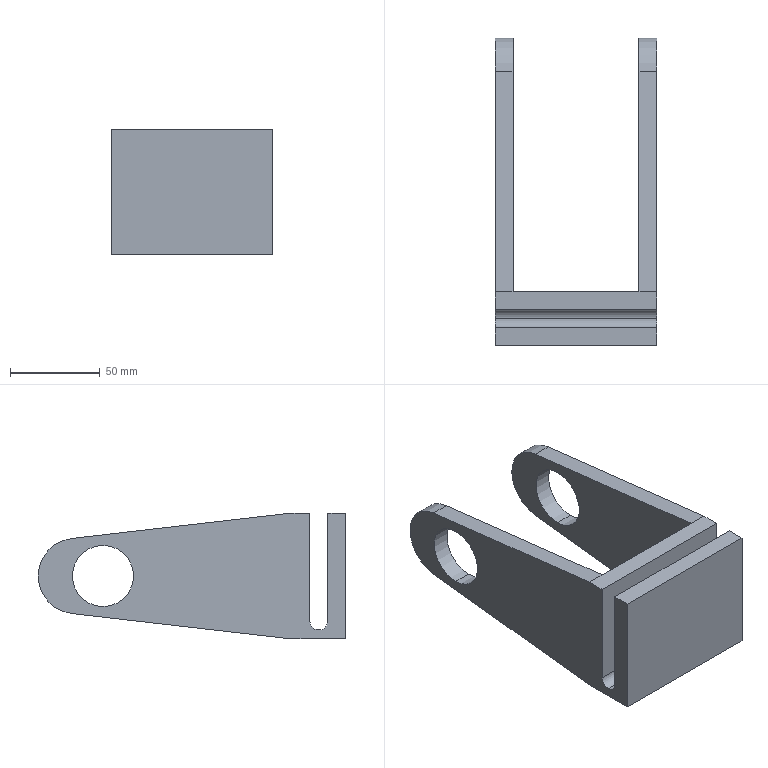Part | SolidWorks | features ICE 2, Extrusion 1, MirrorPattern 1 | 1 solid | 23 faces | box 90 x 171 x 70 mm | volume 261901 mm3 | plane 15 | cylinder 8 | commonest cylinder face diameters 34 x4 10 x2 42 x2
STEP:
#1=CARTESIAN_POINT('',(-45.,15.,-30.));
#2=VERTEX_POINT('',#1);
#3=CARTESIAN_POINT('',(-45.,20.,-25.));
#4=VERTEX_POINT('',#3);
#5=CARTESIAN_POINT('',(-45.,15.,-25.));
#6=DIRECTION('',(1.,0.,0.));
#7=DIRECTION('',(0.,0.,-1.));
#8=AXIS2_PLACEMENT_3D('',#5,#6,#7);
#9=CIRCLE('',#8,5.);
#10=EDGE_CURVE('',#2,#4,#9,.T.);
#11=ORIENTED_EDGE('',*,*,#10,.F.);
#12=CARTESIAN_POINT('',(45.,15.,-30.));
#13=VERTEX_POINT('',#12);
#14=CARTESIAN_POINT('',(-45.,15.,-30.));
#15=DIRECTION('',(1.,0.,0.));
#16=VECTOR('',#15,1000.);
#17=LINE('',#14,#16);
#18=EDGE_CURVE('',#2,#13,#17,.T.);
#19=ORIENTED_EDGE('',*,*,#18,.T.);
#20=CARTESIAN_POINT('',(45.,20.,-25.));
#21=VERTEX_POINT('',#20);
#22=CARTESIAN_POINT('',(45.,15.,-25.));
#23=DIRECTION('',(1.,0.,0.));
#24=DIRECTION('',(0.,0.,-1.));
#25=AXIS2_PLACEMENT_3D('',#22,#23,#24);
#26=CIRCLE('',#25,5.);
#27=EDGE_CURVE('',#13,#21,#26,.T.);
#28=ORIENTED_EDGE('',*,*,#27,.T.);
#29=CARTESIAN_POINT('',(-45.,20.,-25.));
#30=DIRECTION('',(1.,0.,0.));
#31=VECTOR('',#30,1000.);
#32=LINE('',#29,#31);
#33=EDGE_CURVE('',#4,#21,#32,.T.);
#34=ORIENTED_EDGE('',*,*,#33,.F.);
#35=EDGE_LOOP('',(#11,#19,#28,#34));
#36=FACE_OUTER_BOUND('',#35,.T.);
#37=CARTESIAN_POINT('',(-45.,15.,-25.));
#38=DIRECTION('',(1.,0.,0.));
#39=DIRECTION('',(0.,0.,-1.));
#40=AXIS2_PLACEMENT_3D('',#37,#38,#39);
#41=CYLINDRICAL_SURFACE('',#40,5.);
#42=ADVANCED_FACE('',(#36),#41,.F.);
#43=CARTESIAN_POINT('',(-35.,135.,17.));
#44=VERTEX_POINT('',#43);
#45=CARTESIAN_POINT('',(-35.,135.,-17.));
#46=VERTEX_POINT('',#45);
#47=CARTESIAN_POINT('',(-35.,135.,0.));
#48=DIRECTION('',(1.,0.,0.));
#49=DIRECTION('',(0.,0.,-1.));
#50=AXIS2_PLACEMENT_3D('',#47,#48,#49);
#51=CIRCLE('',#50,17.);
#52=EDGE_CURVE('',#44,#46,#51,.T.);
#53=ORIENTED_EDGE('',*,*,#52,.T.);
#54=CARTESIAN_POINT('',(-45.,135.,-17.));
#55=VERTEX_POINT('',#54);
#56=CARTESIAN_POINT('',(-35.,135.,-17.));
#57=DIRECTION('',(-1.,0.,0.));
#58=VECTOR('',#57,1000.);
#59=LINE('',#56,#58);
#60=EDGE_CURVE('',#46,#55,#59,.T.);
#61=ORIENTED_EDGE('',*,*,#60,.T.);
#62=CARTESIAN_POINT('',(-45.,135.,17.));
#63=VERTEX_POINT('',#62);
#64=CARTESIAN_POINT('',(-45.,135.,0.));
#65=DIRECTION('',(1.,0.,0.));
#66=DIRECTION('',(0.,0.,-1.));
#67=AXIS2_PLACEMENT_3D('',#64,#65,#66);
#68=CIRCLE('',#67,17.);
#69=EDGE_CURVE('',#63,#55,#68,.T.);
#70=ORIENTED_EDGE('',*,*,#69,.F.);
#71=CARTESIAN_POINT('',(-35.,135.,17.));
#72=DIRECTION('',(-1.,0.,0.));
#73=VECTOR('',#72,1000.);
#74=LINE('',#71,#73);
#75=EDGE_CURVE('',#44,#63,#74,.T.);
#76=ORIENTED_EDGE('',*,*,#75,.F.);
#77=EDGE_LOOP('',(#53,#61,#70,#76));
#78=FACE_OUTER_BOUND('',#77,.T.);
#79=CARTESIAN_POINT('',(-35.,135.,0.));
#80=DIRECTION('',(-1.,0.,0.));
#81=DIRECTION('',(0.,0.,1.));
#82=AXIS2_PLACEMENT_3D('',#79,#80,#81);
#83=CYLINDRICAL_SURFACE('',#82,17.);
#84=ADVANCED_FACE('',(#78),#83,.F.);
#85=CARTESIAN_POINT('',(35.,135.,17.));
#86=VERTEX_POINT('',#85);
#87=CARTESIAN_POINT('',(35.,135.,-17.));
#88=VERTEX_POINT('',#87);
#89=CARTESIAN_POINT('',(35.,135.,0.));
#90=DIRECTION('',(1.,0.,0.));
#91=DIRECTION('',(0.,0.,-1.));
#92=AXIS2_PLACEMENT_3D('',#89,#90,#91);
#93=CIRCLE('',#92,17.);
#94=EDGE_CURVE('',#86,#88,#93,.T.);
#95=ORIENTED_EDGE('',*,*,#94,.F.);
#96=CARTESIAN_POINT('',(45.,135.,17.));
#97=VERTEX_POINT('',#96);
#98=CARTESIAN_POINT('',(35.,135.,17.));
#99=DIRECTION('',(1.,0.,0.));
#100=VECTOR('',#99,1000.);
#101=LINE('',#98,#100);
#102=EDGE_CURVE('',#86,#97,#101,.T.);
#103=ORIENTED_EDGE('',*,*,#102,.T.);
#104=CARTESIAN_POINT('',(45.,135.,-17.));
#105=VERTEX_POINT('',#104);
#106=CARTESIAN_POINT('',(45.,135.,0.));
#107=DIRECTION('',(1.,0.,0.));
#108=DIRECTION('',(0.,0.,-1.));
#109=AXIS2_PLACEMENT_3D('',#106,#107,#108);
#110=CIRCLE('',#109,17.);
#111=EDGE_CURVE('',#97,#105,#110,.T.);
#112=ORIENTED_EDGE('',*,*,#111,.T.);
#113=CARTESIAN_POINT('',(35.,135.,-17.));
#114=DIRECTION('',(1.,0.,0.));
#115=VECTOR('',#114,1000.);
#116=LINE('',#113,#115);
#117=EDGE_CURVE('',#88,#105,#116,.T.);
#118=ORIENTED_EDGE('',*,*,#117,.F.);
#119=EDGE_LOOP('',(#95,#103,#112,#118));
#120=FACE_OUTER_BOUND('',#119,.T.);
#121=CARTESIAN_POINT('',(35.,135.,0.));
#122=DIRECTION('',(1.,0.,0.));
#123=DIRECTION('',(0.,0.,-1.));
#124=AXIS2_PLACEMENT_3D('',#121,#122,#123);
#125=CYLINDRICAL_SURFACE('',#124,17.);
#126=ADVANCED_FACE('',(#120),#125,.F.);
#127=CARTESIAN_POINT('',(-45.,20.,35.));
#128=VERTEX_POINT('',#127);
#129=CARTESIAN_POINT('',(45.,20.,35.));
#130=VERTEX_POINT('',#129);
#131=CARTESIAN_POINT('',(-45.,20.,35.));
#132=DIRECTION('',(1.,0.,0.));
#133=VECTOR('',#132,1000.);
#134=LINE('',#131,#133);
#135=EDGE_CURVE('',#128,#130,#134,.T.);
#136=ORIENTED_EDGE('',*,*,#135,.T.);
#137=CARTESIAN_POINT('',(45.,30.,35.));
#138=VERTEX_POINT('',#137);
#139=CARTESIAN_POINT('',(45.,30.,35.));
#140=DIRECTION('',(0.,-1.,0.));
#141=VECTOR('',#140,1000.);
#142=LINE('',#139,#141);
#143=EDGE_CURVE('',#138,#130,#142,.T.);
#144=ORIENTED_EDGE('',*,*,#143,.F.);
#145=CARTESIAN_POINT('',(35.,30.,35.));
#146=VERTEX_POINT('',#145);
#147=CARTESIAN_POINT('',(35.,30.,35.));
#148=DIRECTION('',(1.,0.,0.));
#149=VECTOR('',#148,1000.);
#150=LINE('',#147,#149);
#151=EDGE_CURVE('',#146,#138,#150,.T.);
#152=ORIENTED_EDGE('',*,*,#151,.F.);
#153=CARTESIAN_POINT('',(-35.,30.,35.));
#154=VERTEX_POINT('',#153);
#155=CARTESIAN_POINT('',(45.,30.,35.));
#156=DIRECTION('',(1.,0.,0.));
#157=VECTOR('',#156,1000.);
#158=LINE('',#155,#157);
#159=EDGE_CURVE('',#154,#146,#158,.T.);
#160=ORIENTED_EDGE('',*,*,#159,.F.);
#161=CARTESIAN_POINT('',(-45.,30.,35.));
#162=VERTEX_POINT('',#161);
#163=CARTESIAN_POINT('',(45.,30.,35.));
#164=DIRECTION('',(1.,0.,0.));
#165=VECTOR('',#164,1000.);
#166=LINE('',#163,#165);
#167=EDGE_CURVE('',#162,#154,#166,.T.);
#168=ORIENTED_EDGE('',*,*,#167,.F.);
#169=CARTESIAN_POINT('',(-45.,30.,35.));
#170=DIRECTION('',(0.,-1.,0.));
#171=VECTOR('',#170,1000.);
#172=LINE('',#169,#171);
#173=EDGE_CURVE('',#162,#128,#172,.T.);
#174=ORIENTED_EDGE('',*,*,#173,.T.);
#175=EDGE_LOOP('',(#136,#144,#152,#160,#168,#174));
#176=FACE_OUTER_BOUND('',#175,.T.);
#177=CARTESIAN_POINT('',(45.,30.,35.));
#178=DIRECTION('',(0.,0.,-1.));
#179=DIRECTION('',(-1.,0.,0.));
#180=AXIS2_PLACEMENT_3D('',#177,#178,#179);
#181=PLANE('',#180);
#182=ADVANCED_FACE('',(#176),#181,.F.);
#183=CARTESIAN_POINT('',(35.,30.,-35.));
#184=VERTEX_POINT('',#183);
#185=CARTESIAN_POINT('',(-35.,30.,-35.));
#186=VERTEX_POINT('',#185);
#187=CARTESIAN_POINT('',(45.,30.,-35.));
#188=DIRECTION('',(-1.,0.,0.));
#189=VECTOR('',#188,1000.);
#190=LINE('',#187,#189);
#191=EDGE_CURVE('',#184,#186,#190,.T.);
#192=ORIENTED_EDGE('',*,*,#191,.T.);
#193=CARTESIAN_POINT('',(-35.,30.,-35.));
#194=DIRECTION('',(0.,0.,-1.));
#195=VECTOR('',#194,1000.);
#196=LINE('',#193,#195);
#197=EDGE_CURVE('',#154,#186,#196,.T.);
#198=ORIENTED_EDGE('',*,*,#197,.F.);
#199=ORIENTED_EDGE('',*,*,#159,.T.);
#200=CARTESIAN_POINT('',(35.,30.,-35.));
#201=DIRECTION('',(0.,0.,-1.));
#202=VECTOR('',#201,1000.);
#203=LINE('',#200,#202);
#204=EDGE_CURVE('',#146,#184,#203,.T.);
#205=ORIENTED_EDGE('',*,*,#204,.T.);
#206=EDGE_LOOP('',(#192,#198,#199,#205));
#207=FACE_OUTER_BOUND('',#206,.T.);
#208=CARTESIAN_POINT('',(0.,30.,0.));
#209=DIRECTION('',(0.,1.,0.));
#210=DIRECTION('',(0.,0.,1.));
#211=AXIS2_PLACEMENT_3D('',#208,#209,#210);
#212=PLANE('',#211);
#213=ADVANCED_FACE('',(#207),#212,.T.);
#214=CARTESIAN_POINT('',(-45.,10.,35.));
#215=VERTEX_POINT('',#214);
#216=CARTESIAN_POINT('',(-45.,0.,35.));
#217=VERTEX_POINT('',#216);
#218=CARTESIAN_POINT('',(-45.,30.,35.));
#219=DIRECTION('',(0.,-1.,0.));
#220=VECTOR('',#219,1000.);
#221=LINE('',#218,#220);
#222=EDGE_CURVE('',#215,#217,#221,.T.);
#223=ORIENTED_EDGE('',*,*,#222,.F.);
#224=CARTESIAN_POINT('',(-45.,10.,-25.));
#225=VERTEX_POINT('',#224);
#226=CARTESIAN_POINT('',(-45.,10.,35.));
#227=DIRECTION('',(0.,0.,-1.));
#228=VECTOR('',#227,1000.);
#229=LINE('',#226,#228);
#230=EDGE_CURVE('',#215,#225,#229,.T.);
#231=ORIENTED_EDGE('',*,*,#230,.T.);
#232=CARTESIAN_POINT('',(-45.,15.,-25.));
#233=DIRECTION('',(1.,0.,0.));
#234=DIRECTION('',(0.,0.,-1.));
#235=AXIS2_PLACEMENT_3D('',#232,#233,#234);
#236=CIRCLE('',#235,5.);
#237=EDGE_CURVE('',#225,#2,#236,.T.);
#238=ORIENTED_EDGE('',*,*,#237,.T.);
#239=ORIENTED_EDGE('',*,*,#10,.T.);
#240=CARTESIAN_POINT('',(-45.,20.,35.));
#241=DIRECTION('',(0.,0.,-1.));
#242=VECTOR('',#241,1000.);
#243=LINE('',#240,#242);
#244=EDGE_CURVE('',#128,#4,#243,.T.);
#245=ORIENTED_EDGE('',*,*,#244,.F.);
#246=ORIENTED_EDGE('',*,*,#173,.F.);
#247=CARTESIAN_POINT('',(-45.,152.41,20.861));
#248=VERTEX_POINT('',#247);
#249=CARTESIAN_POINT('',(-45.,152.41,20.861));
#250=DIRECTION('',(0.,-0.9934,0.1147));
#251=VECTOR('',#250,1000.);
#252=LINE('',#249,#251);
#253=EDGE_CURVE('',#248,#162,#252,.T.);
#254=ORIENTED_EDGE('',*,*,#253,.F.);
#255=CARTESIAN_POINT('',(-45.,152.41,-20.861));
#256=VERTEX_POINT('',#255);
#257=CARTESIAN_POINT('',(-45.,150.,0.));
#258=DIRECTION('',(1.,0.,0.));
#259=DIRECTION('',(0.,0.,-1.));
#260=AXIS2_PLACEMENT_3D('',#257,#258,#259);
#261=CIRCLE('',#260,21.);
#262=EDGE_CURVE('',#256,#248,#261,.T.);
#263=ORIENTED_EDGE('',*,*,#262,.F.);
#264=CARTESIAN_POINT('',(-45.,30.,-35.));
#265=VERTEX_POINT('',#264);
#266=CARTESIAN_POINT('',(-45.,152.41,-20.861));
#267=DIRECTION('',(0.,0.9934,0.1147));
#268=VECTOR('',#267,1000.);
#269=LINE('',#266,#268);
#270=EDGE_CURVE('',#265,#256,#269,.T.);
#271=ORIENTED_EDGE('',*,*,#270,.F.);
#272=CARTESIAN_POINT('',(-45.,0.,-35.));
#273=VERTEX_POINT('',#272);
#274=CARTESIAN_POINT('',(-45.,30.,-35.));
#275=DIRECTION('',(0.,-1.,0.));
#276=VECTOR('',#275,1000.);
#277=LINE('',#274,#276);
#278=EDGE_CURVE('',#265,#273,#277,.T.);
#279=ORIENTED_EDGE('',*,*,#278,.T.);
#280=CARTESIAN_POINT('',(-45.,0.,35.));
#281=DIRECTION('',(0.,0.,1.));
#282=VECTOR('',#281,1000.);
#283=LINE('',#280,#282);
#284=EDGE_CURVE('',#273,#217,#283,.T.);
#285=ORIENTED_EDGE('',*,*,#284,.T.);
#286=EDGE_LOOP('',(#223,#231,#238,#239,#245,#246,#254,#263,#271,#279,#285));
#287=FACE_OUTER_BOUND('',#286,.T.);
#288=ORIENTED_EDGE('',*,*,#69,.T.);
#289=CARTESIAN_POINT('',(-45.,135.,0.));
#290=DIRECTION('',(1.,0.,0.));
#291=DIRECTION('',(0.,0.,-1.));
#292=AXIS2_PLACEMENT_3D('',#289,#290,#291);
#293=CIRCLE('',#292,17.);
#294=EDGE_CURVE('',#55,#63,#293,.T.);
#295=ORIENTED_EDGE('',*,*,#294,.T.);
#296=EDGE_LOOP('',(#288,#295));
#297=FACE_BOUND('',#296,.T.);
#298=CARTESIAN_POINT('',(-45.,30.,35.));
#299=DIRECTION('',(1.,0.,0.));
#300=DIRECTION('',(0.,0.,-1.));
#301=AXIS2_PLACEMENT_3D('',#298,#299,#300);
#302=PLANE('',#301);
#303=ADVANCED_FACE('',(#287,#297),#302,.F.);
#304=CARTESIAN_POINT('',(45.,10.,35.));
#305=VERTEX_POINT('',#304);
#306=CARTESIAN_POINT('',(45.,0.,35.));
#307=VERTEX_POINT('',#306);
#308=CARTESIAN_POINT('',(45.,30.,35.));
#309=DIRECTION('',(0.,-1.,0.));
#310=VECTOR('',#309,1000.);
#311=LINE('',#308,#310);
#312=EDGE_CURVE('',#305,#307,#311,.T.);
#313=ORIENTED_EDGE('',*,*,#312,.F.);
#314=CARTESIAN_POINT('',(-45.,10.,35.));
#315=DIRECTION('',(1.,0.,0.));
#316=VECTOR('',#315,1000.);
#317=LINE('',#314,#316);
#318=EDGE_CURVE('',#215,#305,#317,.T.);
#319=ORIENTED_EDGE('',*,*,#318,.F.);
#320=ORIENTED_EDGE('',*,*,#222,.T.);
#321=CARTESIAN_POINT('',(45.,0.,35.));
#322=DIRECTION('',(1.,0.,0.));
#323=VECTOR('',#322,1000.);
#324=LINE('',#321,#323);
#325=EDGE_CURVE('',#217,#307,#324,.T.);
#326=ORIENTED_EDGE('',*,*,#325,.T.);
#327=EDGE_LOOP('',(#313,#319,#320,#326));
#328=FACE_OUTER_BOUND('',#327,.T.);
#329=CARTESIAN_POINT('',(45.,30.,35.));
#330=DIRECTION('',(0.,0.,-1.));
#331=DIRECTION('',(-1.,0.,0.));
#332=AXIS2_PLACEMENT_3D('',#329,#330,#331);
#333=PLANE('',#332);
#334=ADVANCED_FACE('',(#328),#333,.F.);
#335=CARTESIAN_POINT('',(45.,10.,-25.));
#336=VERTEX_POINT('',#335);
#337=CARTESIAN_POINT('',(45.,15.,-25.));
#338=DIRECTION('',(1.,0.,0.));
#339=DIRECTION('',(0.,0.,-1.));
#340=AXIS2_PLACEMENT_3D('',#337,#338,#339);
#341=CIRCLE('',#340,5.);
#342=EDGE_CURVE('',#336,#13,#341,.T.);
#343=ORIENTED_EDGE('',*,*,#342,.F.);
#344=CARTESIAN_POINT('',(45.,10.,0.));
#345=DIRECTION('',(0.,0.,-1.));
#346=VECTOR('',#345,1000.);
#347=LINE('',#344,#346);
#348=EDGE_CURVE('',#305,#336,#347,.T.);
#349=ORIENTED_EDGE('',*,*,#348,.F.);
#350=ORIENTED_EDGE('',*,*,#312,.T.);
#351=CARTESIAN_POINT('',(45.,0.,-35.));
#352=VERTEX_POINT('',#351);
#353=CARTESIAN_POINT('',(45.,0.,35.));
#354=DIRECTION('',(0.,0.,-1.));
#355=VECTOR('',#354,1000.);
#356=LINE('',#353,#355);
#357=EDGE_CURVE('',#307,#352,#356,.T.);
#358=ORIENTED_EDGE('',*,*,#357,.T.);
#359=CARTESIAN_POINT('',(45.,30.,-35.));
#360=VERTEX_POINT('',#359);
#361=CARTESIAN_POINT('',(45.,30.,-35.));
#362=DIRECTION('',(0.,-1.,0.));
#363=VECTOR('',#362,1000.);
#364=LINE('',#361,#363);
#365=EDGE_CURVE('',#360,#352,#364,.T.);
#366=ORIENTED_EDGE('',*,*,#365,.F.);
#367=CARTESIAN_POINT('',(45.,152.41,-20.861));
#368=VERTEX_POINT('',#367);
#369=CARTESIAN_POINT('',(45.,152.41,-20.861));
#370=DIRECTION('',(0.,0.9934,0.1147));
#371=VECTOR('',#370,1000.);
#372=LINE('',#369,#371);
#373=EDGE_CURVE('',#360,#368,#372,.T.);
#374=ORIENTED_EDGE('',*,*,#373,.T.);
#375=CARTESIAN_POINT('',(45.,152.41,20.861));
#376=VERTEX_POINT('',#375);
#377=CARTESIAN_POINT('',(45.,150.,0.));
#378=DIRECTION('',(1.,0.,0.));
#379=DIRECTION('',(0.,0.,-1.));
#380=AXIS2_PLACEMENT_3D('',#377,#378,#379);
#381=CIRCLE('',#380,21.);
#382=EDGE_CURVE('',#368,#376,#381,.T.);
#383=ORIENTED_EDGE('',*,*,#382,.T.);
#384=CARTESIAN_POINT('',(45.,152.41,20.861));
#385=DIRECTION('',(0.,-0.9934,0.1147));
#386=VECTOR('',#385,1000.);
#387=LINE('',#384,#386);
#388=EDGE_CURVE('',#376,#138,#387,.T.);
#389=ORIENTED_EDGE('',*,*,#388,.T.);
#390=ORIENTED_EDGE('',*,*,#143,.T.);
#391=CARTESIAN_POINT('',(45.,20.,0.));
#392=DIRECTION('',(0.,0.,-1.));
#393=VECTOR('',#392,1000.);
#394=LINE('',#391,#393);
#395=EDGE_CURVE('',#130,#21,#394,.T.);
#396=ORIENTED_EDGE('',*,*,#395,.T.);
#397=ORIENTED_EDGE('',*,*,#27,.F.);
#398=EDGE_LOOP('',(#343,#349,#350,#358,#366,#374,#383,#389,#390,#396,#397));
#399=FACE_OUTER_BOUND('',#398,.T.);
#400=CARTESIAN_POINT('',(45.,135.,0.));
#401=DIRECTION('',(1.,0.,0.));
#402=DIRECTION('',(0.,0.,-1.));
#403=AXIS2_PLACEMENT_3D('',#400,#401,#402);
#404=CIRCLE('',#403,17.);
#405=EDGE_CURVE('',#105,#97,#404,.T.);
#406=ORIENTED_EDGE('',*,*,#405,.F.);
#407=ORIENTED_EDGE('',*,*,#111,.F.);
#408=EDGE_LOOP('',(#406,#407));
#409=FACE_BOUND('',#408,.T.);
#410=CARTESIAN_POINT('',(45.,30.,35.));
#411=DIRECTION('',(-1.,0.,0.));
#412=DIRECTION('',(0.,0.,1.));
#413=AXIS2_PLACEMENT_3D('',#410,#411,#412);
#414=PLANE('',#413);
#415=ADVANCED_FACE('',(#399,#409),#414,.F.);
#416=CARTESIAN_POINT('',(45.,0.,-35.));
#417=DIRECTION('',(-1.,0.,0.));
#418=VECTOR('',#417,1000.);
#419=LINE('',#416,#418);
#420=EDGE_CURVE('',#352,#273,#419,.T.);
#421=ORIENTED_EDGE('',*,*,#420,.T.);
#422=ORIENTED_EDGE('',*,*,#278,.F.);
#423=CARTESIAN_POINT('',(-35.,30.,-35.));
#424=DIRECTION('',(-1.,0.,0.));
#425=VECTOR('',#424,1000.);
#426=LINE('',#423,#425);
#427=EDGE_CURVE('',#186,#265,#426,.T.);
#428=ORIENTED_EDGE('',*,*,#427,.F.);
#429=ORIENTED_EDGE('',*,*,#191,.F.);
#430=CARTESIAN_POINT('',(45.,30.,-35.));
#431=DIRECTION('',(-1.,0.,0.));
#432=VECTOR('',#431,1000.);
#433=LINE('',#430,#432);
#434=EDGE_CURVE('',#360,#184,#433,.T.);
#435=ORIENTED_EDGE('',*,*,#434,.F.);
#436=ORIENTED_EDGE('',*,*,#365,.T.);
#437=EDGE_LOOP('',(#421,#422,#428,#429,#435,#436));
#438=FACE_OUTER_BOUND('',#437,.T.);
#439=CARTESIAN_POINT('',(45.,30.,-35.));
#440=DIRECTION('',(0.,0.,1.));
#441=DIRECTION('',(1.,0.,0.));
#442=AXIS2_PLACEMENT_3D('',#439,#440,#441);
#443=PLANE('',#442);
#444=ADVANCED_FACE('',(#438),#443,.F.);
#445=ORIENTED_EDGE('',*,*,#284,.F.);
#446=ORIENTED_EDGE('',*,*,#420,.F.);
#447=ORIENTED_EDGE('',*,*,#357,.F.);
#448=ORIENTED_EDGE('',*,*,#325,.F.);
#449=EDGE_LOOP('',(#445,#446,#447,#448));
#450=FACE_OUTER_BOUND('',#449,.T.);
#451=CARTESIAN_POINT('',(0.,0.,0.));
#452=DIRECTION('',(0.,1.,0.));
#453=DIRECTION('',(0.,0.,1.));
#454=AXIS2_PLACEMENT_3D('',#451,#452,#453);
#455=PLANE('',#454);
#456=ADVANCED_FACE('',(#450),#455,.F.);
#457=ORIENTED_EDGE('',*,*,#382,.F.);
#458=CARTESIAN_POINT('',(35.,152.41,-20.861));
#459=VERTEX_POINT('',#458);
#460=CARTESIAN_POINT('',(35.,152.41,-20.861));
#461=DIRECTION('',(1.,0.,0.));
#462=VECTOR('',#461,1000.);
#463=LINE('',#460,#462);
#464=EDGE_CURVE('',#459,#368,#463,.T.);
#465=ORIENTED_EDGE('',*,*,#464,.F.);
#466=CARTESIAN_POINT('',(35.,152.41,20.861));
#467=VERTEX_POINT('',#466);
#468=CARTESIAN_POINT('',(35.,150.,0.));
#469=DIRECTION('',(1.,0.,0.));
#470=DIRECTION('',(0.,0.,-1.));
#471=AXIS2_PLACEMENT_3D('',#468,#469,#470);
#472=CIRCLE('',#471,21.);
#473=EDGE_CURVE('',#459,#467,#472,.T.);
#474=ORIENTED_EDGE('',*,*,#473,.T.);
#475=CARTESIAN_POINT('',(35.,152.41,20.861));
#476=DIRECTION('',(1.,0.,0.));
#477=VECTOR('',#476,1000.);
#478=LINE('',#475,#477);
#479=EDGE_CURVE('',#467,#376,#478,.T.);
#480=ORIENTED_EDGE('',*,*,#479,.T.);
#481=EDGE_LOOP('',(#457,#465,#474,#480));
#482=FACE_OUTER_BOUND('',#481,.T.);
#483=CARTESIAN_POINT('',(35.,150.,0.));
#484=DIRECTION('',(1.,0.,0.));
#485=DIRECTION('',(0.,0.,-1.));
#486=AXIS2_PLACEMENT_3D('',#483,#484,#485);
#487=CYLINDRICAL_SURFACE('',#486,21.);
#488=ADVANCED_FACE('',(#482),#487,.T.);
#489=ORIENTED_EDGE('',*,*,#373,.F.);
#490=ORIENTED_EDGE('',*,*,#434,.T.);
#491=CARTESIAN_POINT('',(35.,152.41,-20.861));
#492=DIRECTION('',(0.,0.9934,0.1147));
#493=VECTOR('',#492,1000.);
#494=LINE('',#491,#493);
#495=EDGE_CURVE('',#184,#459,#494,.T.);
#496=ORIENTED_EDGE('',*,*,#495,.T.);
#497=ORIENTED_EDGE('',*,*,#464,.T.);
#498=EDGE_LOOP('',(#489,#490,#496,#497));
#499=FACE_OUTER_BOUND('',#498,.T.);
#500=CARTESIAN_POINT('',(35.,152.41,-20.861));
#501=DIRECTION('',(0.,0.1147,-0.9934));
#502=DIRECTION('',(0.,0.9934,0.1147));
#503=AXIS2_PLACEMENT_3D('',#500,#501,#502);
#504=PLANE('',#503);
#505=ADVANCED_FACE('',(#499),#504,.T.);
#506=ORIENTED_EDGE('',*,*,#388,.F.);
#507=ORIENTED_EDGE('',*,*,#479,.F.);
#508=CARTESIAN_POINT('',(35.,152.41,20.861));
#509=DIRECTION('',(0.,-0.9934,0.1147));
#510=VECTOR('',#509,1000.);
#511=LINE('',#508,#510);
#512=EDGE_CURVE('',#467,#146,#511,.T.);
#513=ORIENTED_EDGE('',*,*,#512,.T.);
#514=ORIENTED_EDGE('',*,*,#151,.T.);
#515=EDGE_LOOP('',(#506,#507,#513,#514));
#516=FACE_OUTER_BOUND('',#515,.T.);
#517=CARTESIAN_POINT('',(35.,152.41,20.861));
#518=DIRECTION('',(0.,0.1147,0.9934));
#519=DIRECTION('',(0.,-0.9934,0.1147));
#520=AXIS2_PLACEMENT_3D('',#517,#518,#519);
#521=PLANE('',#520);
#522=ADVANCED_FACE('',(#516),#521,.T.);
#523=CARTESIAN_POINT('',(35.,135.,0.));
#524=DIRECTION('',(1.,0.,0.));
#525=DIRECTION('',(0.,0.,-1.));
#526=AXIS2_PLACEMENT_3D('',#523,#524,#525);
#527=CIRCLE('',#526,17.);
#528=EDGE_CURVE('',#88,#86,#527,.T.);
#529=ORIENTED_EDGE('',*,*,#528,.T.);
#530=ORIENTED_EDGE('',*,*,#94,.T.);
#531=EDGE_LOOP('',(#529,#530));
#532=FACE_BOUND('',#531,.T.);
#533=ORIENTED_EDGE('',*,*,#473,.F.);
#534=ORIENTED_EDGE('',*,*,#495,.F.);
#535=ORIENTED_EDGE('',*,*,#204,.F.);
#536=ORIENTED_EDGE('',*,*,#512,.F.);
#537=EDGE_LOOP('',(#533,#534,#535,#536));
#538=FACE_OUTER_BOUND('',#537,.T.);
#539=CARTESIAN_POINT('',(35.,150.,0.));
#540=DIRECTION('',(1.,0.,0.));
#541=DIRECTION('',(0.,0.,-1.));
#542=AXIS2_PLACEMENT_3D('',#539,#540,#541);
#543=PLANE('',#542);
#544=ADVANCED_FACE('',(#532,#538),#543,.F.);
#545=ORIENTED_EDGE('',*,*,#102,.F.);
#546=ORIENTED_EDGE('',*,*,#528,.F.);
#547=ORIENTED_EDGE('',*,*,#117,.T.);
#548=ORIENTED_EDGE('',*,*,#405,.T.);
#549=EDGE_LOOP('',(#545,#546,#547,#548));
#550=FACE_OUTER_BOUND('',#549,.T.);
#551=CARTESIAN_POINT('',(35.,135.,0.));
#552=DIRECTION('',(1.,0.,0.));
#553=DIRECTION('',(0.,0.,-1.));
#554=AXIS2_PLACEMENT_3D('',#551,#552,#553);
#555=CYLINDRICAL_SURFACE('',#554,17.);
#556=ADVANCED_FACE('',(#550),#555,.F.);
#557=CARTESIAN_POINT('',(-35.,152.41,-20.861));
#558=VERTEX_POINT('',#557);
#559=CARTESIAN_POINT('',(-35.,152.41,20.861));
#560=VERTEX_POINT('',#559);
#561=CARTESIAN_POINT('',(-35.,150.,0.));
#562=DIRECTION('',(1.,0.,0.));
#563=DIRECTION('',(0.,0.,-1.));
#564=AXIS2_PLACEMENT_3D('',#561,#562,#563);
#565=CIRCLE('',#564,21.);
#566=EDGE_CURVE('',#558,#560,#565,.T.);
#567=ORIENTED_EDGE('',*,*,#566,.T.);
#568=CARTESIAN_POINT('',(-35.,152.41,20.861));
#569=DIRECTION('',(0.,-0.9934,0.1147));
#570=VECTOR('',#569,1000.);
#571=LINE('',#568,#570);
#572=EDGE_CURVE('',#560,#154,#571,.T.);
#573=ORIENTED_EDGE('',*,*,#572,.T.);
#574=ORIENTED_EDGE('',*,*,#197,.T.);
#575=CARTESIAN_POINT('',(-35.,152.41,-20.861));
#576=DIRECTION('',(0.,0.9934,0.1147));
#577=VECTOR('',#576,1000.);
#578=LINE('',#575,#577);
#579=EDGE_CURVE('',#186,#558,#578,.T.);
#580=ORIENTED_EDGE('',*,*,#579,.T.);
#581=EDGE_LOOP('',(#567,#573,#574,#580));
#582=FACE_OUTER_BOUND('',#581,.T.);
#583=ORIENTED_EDGE('',*,*,#52,.F.);
#584=CARTESIAN_POINT('',(-35.,135.,0.));
#585=DIRECTION('',(1.,0.,0.));
#586=DIRECTION('',(0.,0.,-1.));
#587=AXIS2_PLACEMENT_3D('',#584,#585,#586);
#588=CIRCLE('',#587,17.);
#589=EDGE_CURVE('',#46,#44,#588,.T.);
#590=ORIENTED_EDGE('',*,*,#589,.F.);
#591=EDGE_LOOP('',(#583,#590));
#592=FACE_BOUND('',#591,.T.);
#593=CARTESIAN_POINT('',(-35.,150.,0.));
#594=DIRECTION('',(-1.,0.,0.));
#595=DIRECTION('',(0.,0.,-1.));
#596=AXIS2_PLACEMENT_3D('',#593,#594,#595);
#597=PLANE('',#596);
#598=ADVANCED_FACE('',(#582,#592),#597,.F.);
#599=ORIENTED_EDGE('',*,*,#262,.T.);
#600=CARTESIAN_POINT('',(-35.,152.41,20.861));
#601=DIRECTION('',(-1.,0.,0.));
#602=VECTOR('',#601,1000.);
#603=LINE('',#600,#602);
#604=EDGE_CURVE('',#560,#248,#603,.T.);
#605=ORIENTED_EDGE('',*,*,#604,.F.);
#606=ORIENTED_EDGE('',*,*,#566,.F.);
#607=CARTESIAN_POINT('',(-35.,152.41,-20.861));
#608=DIRECTION('',(-1.,0.,0.));
#609=VECTOR('',#608,1000.);
#610=LINE('',#607,#609);
#611=EDGE_CURVE('',#558,#256,#610,.T.);
#612=ORIENTED_EDGE('',*,*,#611,.T.);
#613=EDGE_LOOP('',(#599,#605,#606,#612));
#614=FACE_OUTER_BOUND('',#613,.T.);
#615=CARTESIAN_POINT('',(-35.,150.,0.));
#616=DIRECTION('',(-1.,0.,0.));
#617=DIRECTION('',(0.,0.,1.));
#618=AXIS2_PLACEMENT_3D('',#615,#616,#617);
#619=CYLINDRICAL_SURFACE('',#618,21.);
#620=ADVANCED_FACE('',(#614),#619,.T.);
#621=ORIENTED_EDGE('',*,*,#253,.T.);
#622=ORIENTED_EDGE('',*,*,#167,.T.);
#623=ORIENTED_EDGE('',*,*,#572,.F.);
#624=ORIENTED_EDGE('',*,*,#604,.T.);
#625=EDGE_LOOP('',(#621,#622,#623,#624));
#626=FACE_OUTER_BOUND('',#625,.T.);
#627=CARTESIAN_POINT('',(-35.,152.41,20.861));
#628=DIRECTION('',(0.,-0.1147,-0.9934));
#629=DIRECTION('',(0.,0.9934,-0.1147));
#630=AXIS2_PLACEMENT_3D('',#627,#628,#629);
#631=PLANE('',#630);
#632=ADVANCED_FACE('',(#626),#631,.F.);
#633=ORIENTED_EDGE('',*,*,#270,.T.);
#634=ORIENTED_EDGE('',*,*,#611,.F.);
#635=ORIENTED_EDGE('',*,*,#579,.F.);
#636=ORIENTED_EDGE('',*,*,#427,.T.);
#637=EDGE_LOOP('',(#633,#634,#635,#636));
#638=FACE_OUTER_BOUND('',#637,.T.);
#639=CARTESIAN_POINT('',(-35.,152.41,-20.861));
#640=DIRECTION('',(0.,-0.1147,0.9934));
#641=DIRECTION('',(0.,-0.9934,-0.1147));
#642=AXIS2_PLACEMENT_3D('',#639,#640,#641);
#643=PLANE('',#642);
#644=ADVANCED_FACE('',(#638),#643,.F.);
#645=ORIENTED_EDGE('',*,*,#60,.F.);
#646=ORIENTED_EDGE('',*,*,#589,.T.);
#647=ORIENTED_EDGE('',*,*,#75,.T.);
#648=ORIENTED_EDGE('',*,*,#294,.F.);
#649=EDGE_LOOP('',(#645,#646,#647,#648));
#650=FACE_OUTER_BOUND('',#649,.T.);
#651=CARTESIAN_POINT('',(-35.,135.,0.));
#652=DIRECTION('',(-1.,0.,0.));
#653=DIRECTION('',(0.,0.,1.));
#654=AXIS2_PLACEMENT_3D('',#651,#652,#653);
#655=CYLINDRICAL_SURFACE('',#654,17.);
#656=ADVANCED_FACE('',(#650),#655,.F.);
#657=ORIENTED_EDGE('',*,*,#318,.T.);
#658=ORIENTED_EDGE('',*,*,#348,.T.);
#659=CARTESIAN_POINT('',(-45.,10.,-25.));
#660=DIRECTION('',(1.,0.,0.));
#661=VECTOR('',#660,1000.);
#662=LINE('',#659,#661);
#663=EDGE_CURVE('',#225,#336,#662,.T.);
#664=ORIENTED_EDGE('',*,*,#663,.F.);
#665=ORIENTED_EDGE('',*,*,#230,.F.);
#666=EDGE_LOOP('',(#657,#658,#664,#665));
#667=FACE_OUTER_BOUND('',#666,.T.);
#668=CARTESIAN_POINT('',(-45.,10.,0.));
#669=DIRECTION('',(0.,-1.,0.));
#670=DIRECTION('',(0.,0.,-1.));
#671=AXIS2_PLACEMENT_3D('',#668,#669,#670);
#672=PLANE('',#671);
#673=ADVANCED_FACE('',(#667),#672,.F.);
#674=ORIENTED_EDGE('',*,*,#244,.T.);
#675=ORIENTED_EDGE('',*,*,#33,.T.);
#676=ORIENTED_EDGE('',*,*,#395,.F.);
#677=ORIENTED_EDGE('',*,*,#135,.F.);
#678=EDGE_LOOP('',(#674,#675,#676,#677));
#679=FACE_OUTER_BOUND('',#678,.T.);
#680=CARTESIAN_POINT('',(-45.,20.,0.));
#681=DIRECTION('',(0.,-1.,0.));
#682=DIRECTION('',(0.,0.,-1.));
#683=AXIS2_PLACEMENT_3D('',#680,#681,#682);
#684=PLANE('',#683);
#685=ADVANCED_FACE('',(#679),#684,.T.);
#686=ORIENTED_EDGE('',*,*,#18,.F.);
#687=ORIENTED_EDGE('',*,*,#237,.F.);
#688=ORIENTED_EDGE('',*,*,#663,.T.);
#689=ORIENTED_EDGE('',*,*,#342,.T.);
#690=EDGE_LOOP('',(#686,#687,#688,#689));
#691=FACE_OUTER_BOUND('',#690,.T.);
#692=CARTESIAN_POINT('',(-45.,15.,-25.));
#693=DIRECTION('',(1.,0.,0.));
#694=DIRECTION('',(0.,0.,-1.));
#695=AXIS2_PLACEMENT_3D('',#692,#693,#694);
#696=CYLINDRICAL_SURFACE('',#695,5.);
#697=ADVANCED_FACE('',(#691),#696,.F.);
#698=CLOSED_SHELL('',(#42,#84,#126,#182,#213,#303,#334,#415,#444,#456,#488,#505,#522,#544,#556,#598,#620,#632,#644,#656,#673,#685,#697));
#699=MANIFOLD_SOLID_BREP('',#698);
#700=CARTESIAN_POINT('',(0.,0.,0.));
#701=DIRECTION('',(0.,0.,1.));
#702=DIRECTION('',(1.,0.,0.));
#703=AXIS2_PLACEMENT_3D('',#700,#701,#702);
#704=(LENGTH_UNIT()NAMED_UNIT(*)SI_UNIT(.MILLI.,.METRE.));
#705=UNCERTAINTY_MEASURE_WITH_UNIT(LENGTH_MEASURE(0.00001),#704,'','');
#706=(NAMED_UNIT(*)PLANE_ANGLE_UNIT()SI_UNIT($,.RADIAN.));
#707=(NAMED_UNIT(*)SI_UNIT($,.STERADIAN.)SOLID_ANGLE_UNIT());
#708=(GEOMETRIC_REPRESENTATION_CONTEXT(3)GLOBAL_UNCERTAINTY_ASSIGNED_CONTEXT((#705))GLOBAL_UNIT_ASSIGNED_CONTEXT((#704,#706,#707))REPRESENTATION_CONTEXT('',''));
#709=ADVANCED_BREP_SHAPE_REPRESENTATION('',(#699,#703),#708);